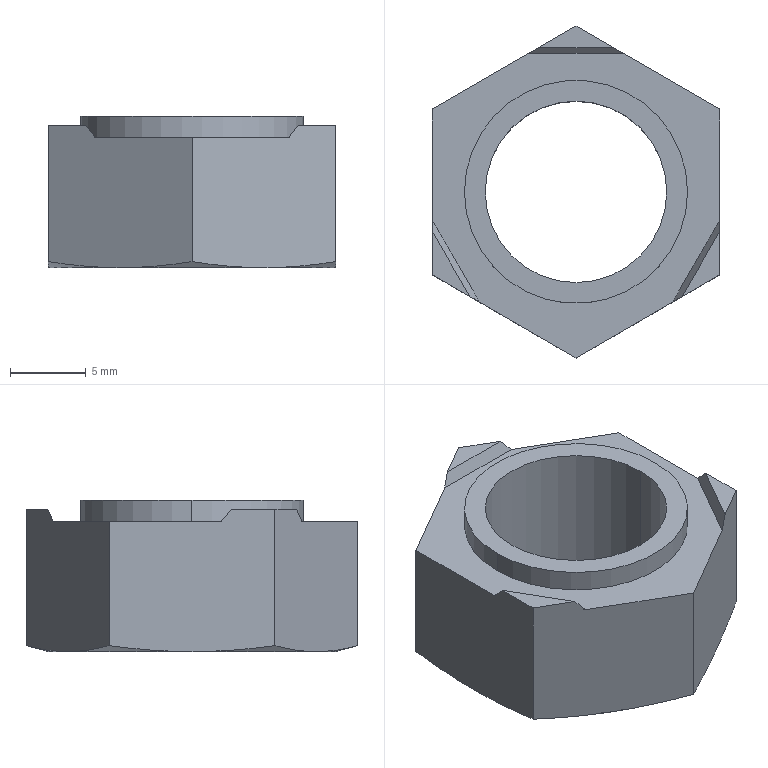Part | SolidWorks | features Cut 3, Boss 1, CirPattern 1, Extrusion 1, RefAxis 1 | 1 solid | 28 faces | box 19 x 21.939 x 10 mm | volume 1791 mm3 | plane 16 | cylinder 6 | cone 6 | commonest cylinder face diameters 12 x2 14.75 x2 15.07 x2
STEP:
#1=CARTESIAN_POINT('',(7.535,0.,0.2));
#2=VERTEX_POINT('',#1);
#3=CARTESIAN_POINT('',(-7.535,0.,0.2));
#4=VERTEX_POINT('',#3);
#5=CARTESIAN_POINT('',(0.,0.,0.2));
#6=DIRECTION('',(0.,0.,-1.));
#7=DIRECTION('',(-1.,0.,0.));
#8=AXIS2_PLACEMENT_3D('',#5,#6,#7);
#9=CIRCLE('',#8,7.535);
#10=EDGE_CURVE('',#2,#4,#9,.T.);
#11=ORIENTED_EDGE('',*,*,#10,.F.);
#12=CARTESIAN_POINT('',(7.535,0.,0.));
#13=VERTEX_POINT('',#12);
#14=CARTESIAN_POINT('',(7.535,0.,0.2));
#15=DIRECTION('',(0.,0.,-1.));
#16=VECTOR('',#15,1000.);
#17=LINE('',#14,#16);
#18=EDGE_CURVE('',#2,#13,#17,.T.);
#19=ORIENTED_EDGE('',*,*,#18,.T.);
#20=CARTESIAN_POINT('',(-7.535,0.,0.));
#21=VERTEX_POINT('',#20);
#22=CARTESIAN_POINT('',(0.,0.,0.));
#23=DIRECTION('',(0.,0.,-1.));
#24=DIRECTION('',(-1.,0.,0.));
#25=AXIS2_PLACEMENT_3D('',#22,#23,#24);
#26=CIRCLE('',#25,7.535);
#27=EDGE_CURVE('',#13,#21,#26,.T.);
#28=ORIENTED_EDGE('',*,*,#27,.T.);
#29=CARTESIAN_POINT('',(-7.535,0.,0.2));
#30=DIRECTION('',(0.,0.,-1.));
#31=VECTOR('',#30,1000.);
#32=LINE('',#29,#31);
#33=EDGE_CURVE('',#4,#21,#32,.T.);
#34=ORIENTED_EDGE('',*,*,#33,.F.);
#35=EDGE_LOOP('',(#11,#19,#28,#34));
#36=FACE_OUTER_BOUND('',#35,.T.);
#37=CARTESIAN_POINT('',(0.,0.,0.2));
#38=DIRECTION('',(0.,0.,-1.));
#39=DIRECTION('',(-1.,0.,0.));
#40=AXIS2_PLACEMENT_3D('',#37,#38,#39);
#41=CYLINDRICAL_SURFACE('',#40,7.535);
#42=ADVANCED_FACE('',(#36),#41,.F.);
#43=CARTESIAN_POINT('',(7.375,0.,10.));
#44=VERTEX_POINT('',#43);
#45=CARTESIAN_POINT('',(-7.375,0.,10.));
#46=VERTEX_POINT('',#45);
#47=CARTESIAN_POINT('',(0.,0.,10.));
#48=DIRECTION('',(0.,0.,1.));
#49=DIRECTION('',(1.,0.,0.));
#50=AXIS2_PLACEMENT_3D('',#47,#48,#49);
#51=CIRCLE('',#50,7.375);
#52=EDGE_CURVE('',#44,#46,#51,.T.);
#53=ORIENTED_EDGE('',*,*,#52,.F.);
#54=CARTESIAN_POINT('',(7.375,0.,8.6));
#55=VERTEX_POINT('',#54);
#56=CARTESIAN_POINT('',(7.375,0.,10.));
#57=DIRECTION('',(0.,0.,-1.));
#58=VECTOR('',#57,1000.);
#59=LINE('',#56,#58);
#60=EDGE_CURVE('',#44,#55,#59,.T.);
#61=ORIENTED_EDGE('',*,*,#60,.T.);
#62=CARTESIAN_POINT('',(-7.375,0.,8.6));
#63=VERTEX_POINT('',#62);
#64=CARTESIAN_POINT('',(0.,0.,8.6));
#65=DIRECTION('',(0.,0.,1.));
#66=DIRECTION('',(-1.,0.,0.));
#67=AXIS2_PLACEMENT_3D('',#64,#65,#66);
#68=CIRCLE('',#67,7.375);
#69=EDGE_CURVE('',#55,#63,#68,.T.);
#70=ORIENTED_EDGE('',*,*,#69,.T.);
#71=CARTESIAN_POINT('',(-7.375,0.,10.));
#72=DIRECTION('',(0.,0.,-1.));
#73=VECTOR('',#72,1000.);
#74=LINE('',#71,#73);
#75=EDGE_CURVE('',#46,#63,#74,.T.);
#76=ORIENTED_EDGE('',*,*,#75,.F.);
#77=EDGE_LOOP('',(#53,#61,#70,#76));
#78=FACE_OUTER_BOUND('',#77,.T.);
#79=CARTESIAN_POINT('',(0.,0.,10.));
#80=DIRECTION('',(0.,0.,-1.));
#81=DIRECTION('',(-1.,0.,0.));
#82=AXIS2_PLACEMENT_3D('',#79,#80,#81);
#83=CYLINDRICAL_SURFACE('',#82,7.375);
#84=ADVANCED_FACE('',(#78),#83,.T.);
#85=CARTESIAN_POINT('',(-6.,0.,10.));
#86=VERTEX_POINT('',#85);
#87=CARTESIAN_POINT('',(6.,0.,10.));
#88=VERTEX_POINT('',#87);
#89=CARTESIAN_POINT('',(0.,0.,10.));
#90=DIRECTION('',(0.,0.,1.));
#91=DIRECTION('',(1.,0.,0.));
#92=AXIS2_PLACEMENT_3D('',#89,#90,#91);
#93=CIRCLE('',#92,6.);
#94=EDGE_CURVE('',#86,#88,#93,.T.);
#95=ORIENTED_EDGE('',*,*,#94,.T.);
#96=CARTESIAN_POINT('',(6.,0.,0.2));
#97=VERTEX_POINT('',#96);
#98=CARTESIAN_POINT('',(6.,0.,10.));
#99=DIRECTION('',(0.,0.,-1.));
#100=VECTOR('',#99,1000.);
#101=LINE('',#98,#100);
#102=EDGE_CURVE('',#88,#97,#101,.T.);
#103=ORIENTED_EDGE('',*,*,#102,.T.);
#104=CARTESIAN_POINT('',(-6.,0.,0.2));
#105=VERTEX_POINT('',#104);
#106=CARTESIAN_POINT('',(0.,0.,0.2));
#107=DIRECTION('',(0.,0.,-1.));
#108=DIRECTION('',(-1.,0.,0.));
#109=AXIS2_PLACEMENT_3D('',#106,#107,#108);
#110=CIRCLE('',#109,6.);
#111=EDGE_CURVE('',#97,#105,#110,.T.);
#112=ORIENTED_EDGE('',*,*,#111,.T.);
#113=CARTESIAN_POINT('',(-6.,0.,10.));
#114=DIRECTION('',(0.,0.,-1.));
#115=VECTOR('',#114,1000.);
#116=LINE('',#113,#115);
#117=EDGE_CURVE('',#86,#105,#116,.T.);
#118=ORIENTED_EDGE('',*,*,#117,.F.);
#119=EDGE_LOOP('',(#95,#103,#112,#118));
#120=FACE_OUTER_BOUND('',#119,.T.);
#121=CARTESIAN_POINT('',(0.,0.,10.));
#122=DIRECTION('',(0.,0.,-1.));
#123=DIRECTION('',(-1.,0.,0.));
#124=AXIS2_PLACEMENT_3D('',#121,#122,#123);
#125=CYLINDRICAL_SURFACE('',#124,6.);
#126=ADVANCED_FACE('',(#120),#125,.F.);
#127=ORIENTED_EDGE('',*,*,#102,.F.);
#128=CARTESIAN_POINT('',(0.,0.,10.));
#129=DIRECTION('',(0.,0.,1.));
#130=DIRECTION('',(1.,0.,0.));
#131=AXIS2_PLACEMENT_3D('',#128,#129,#130);
#132=CIRCLE('',#131,6.);
#133=EDGE_CURVE('',#88,#86,#132,.T.);
#134=ORIENTED_EDGE('',*,*,#133,.T.);
#135=ORIENTED_EDGE('',*,*,#117,.T.);
#136=CARTESIAN_POINT('',(0.,0.,0.2));
#137=DIRECTION('',(0.,0.,-1.));
#138=DIRECTION('',(-1.,0.,0.));
#139=AXIS2_PLACEMENT_3D('',#136,#137,#138);
#140=CIRCLE('',#139,6.);
#141=EDGE_CURVE('',#105,#97,#140,.T.);
#142=ORIENTED_EDGE('',*,*,#141,.T.);
#143=EDGE_LOOP('',(#127,#134,#135,#142));
#144=FACE_OUTER_BOUND('',#143,.T.);
#145=CARTESIAN_POINT('',(0.,0.,10.));
#146=DIRECTION('',(0.,0.,-1.));
#147=DIRECTION('',(-1.,0.,0.));
#148=AXIS2_PLACEMENT_3D('',#145,#146,#147);
#149=CYLINDRICAL_SURFACE('',#148,6.);
#150=ADVANCED_FACE('',(#144),#149,.F.);
#151=CARTESIAN_POINT('',(0.,0.,0.));
#152=DIRECTION('',(0.,0.,-1.));
#153=DIRECTION('',(-1.,0.,0.));
#154=AXIS2_PLACEMENT_3D('',#151,#152,#153);
#155=CIRCLE('',#154,7.535);
#156=EDGE_CURVE('',#21,#13,#155,.T.);
#157=ORIENTED_EDGE('',*,*,#156,.F.);
#158=ORIENTED_EDGE('',*,*,#27,.F.);
#159=EDGE_LOOP('',(#157,#158));
#160=FACE_BOUND('',#159,.T.);
#161=CARTESIAN_POINT('',(4.75,8.227,0.));
#162=VERTEX_POINT('',#161);
#163=CARTESIAN_POINT('',(9.5,0.,0.));
#164=VERTEX_POINT('',#163);
#165=CARTESIAN_POINT('',(0.,0.,0.));
#166=DIRECTION('',(0.,0.,-1.));
#167=DIRECTION('',(-1.,0.,0.));
#168=AXIS2_PLACEMENT_3D('',#165,#166,#167);
#169=CIRCLE('',#168,9.5);
#170=EDGE_CURVE('',#162,#164,#169,.T.);
#171=ORIENTED_EDGE('',*,*,#170,.T.);
#172=CARTESIAN_POINT('',(4.75,-8.227,0.));
#173=VERTEX_POINT('',#172);
#174=CARTESIAN_POINT('',(0.,0.,0.));
#175=DIRECTION('',(0.,0.,-1.));
#176=DIRECTION('',(-1.,0.,0.));
#177=AXIS2_PLACEMENT_3D('',#174,#175,#176);
#178=CIRCLE('',#177,9.5);
#179=EDGE_CURVE('',#164,#173,#178,.T.);
#180=ORIENTED_EDGE('',*,*,#179,.T.);
#181=CARTESIAN_POINT('',(-4.75,-8.227,0.));
#182=VERTEX_POINT('',#181);
#183=CARTESIAN_POINT('',(0.,0.,0.));
#184=DIRECTION('',(0.,0.,-1.));
#185=DIRECTION('',(-1.,0.,0.));
#186=AXIS2_PLACEMENT_3D('',#183,#184,#185);
#187=CIRCLE('',#186,9.5);
#188=EDGE_CURVE('',#173,#182,#187,.T.);
#189=ORIENTED_EDGE('',*,*,#188,.T.);
#190=CARTESIAN_POINT('',(-9.5,0.,0.));
#191=VERTEX_POINT('',#190);
#192=CARTESIAN_POINT('',(0.,0.,0.));
#193=DIRECTION('',(0.,0.,-1.));
#194=DIRECTION('',(-1.,0.,0.));
#195=AXIS2_PLACEMENT_3D('',#192,#193,#194);
#196=CIRCLE('',#195,9.5);
#197=EDGE_CURVE('',#182,#191,#196,.T.);
#198=ORIENTED_EDGE('',*,*,#197,.T.);
#199=CARTESIAN_POINT('',(-4.75,8.227,0.));
#200=VERTEX_POINT('',#199);
#201=CARTESIAN_POINT('',(0.,0.,0.));
#202=DIRECTION('',(0.,0.,-1.));
#203=DIRECTION('',(-1.,0.,0.));
#204=AXIS2_PLACEMENT_3D('',#201,#202,#203);
#205=CIRCLE('',#204,9.5);
#206=EDGE_CURVE('',#191,#200,#205,.T.);
#207=ORIENTED_EDGE('',*,*,#206,.T.);
#208=CARTESIAN_POINT('',(0.,0.,0.));
#209=DIRECTION('',(0.,0.,-1.));
#210=DIRECTION('',(-1.,0.,0.));
#211=AXIS2_PLACEMENT_3D('',#208,#209,#210);
#212=CIRCLE('',#211,9.5);
#213=EDGE_CURVE('',#200,#162,#212,.T.);
#214=ORIENTED_EDGE('',*,*,#213,.T.);
#215=EDGE_LOOP('',(#171,#180,#189,#198,#207,#214));
#216=FACE_OUTER_BOUND('',#215,.T.);
#217=CARTESIAN_POINT('',(-9.5,16.454,0.));
#218=DIRECTION('',(0.,0.,1.));
#219=DIRECTION('',(1.,0.,0.));
#220=AXIS2_PLACEMENT_3D('',#217,#218,#219);
#221=PLANE('',#220);
#222=ADVANCED_FACE('',(#160,#216),#221,.F.);
#223=CARTESIAN_POINT('',(0.,10.97,0.3938));
#224=VERTEX_POINT('',#223);
#225=CARTESIAN_POINT('',(0.,10.97,0.3938));
#226=CARTESIAN_POINT('',(0.7917,10.513,0.2713));
#227=CARTESIAN_POINT('',(1.583,10.056,0.1719));
#228=CARTESIAN_POINT('',(3.167,9.141,0.03601));
#229=CARTESIAN_POINT('',(3.958,8.684,0.));
#230=CARTESIAN_POINT('',(4.75,8.227,0.));
#231=B_SPLINE_CURVE_WITH_KNOTS('',3,(#225,#226,#227,#228,#229,#230),.UNSPECIFIED.,.F.,.F.,(4,2,4),(0.000000231,0.002743,0.005485),.UNSPECIFIED.);
#232=EDGE_CURVE('',#224,#162,#231,.T.);
#233=ORIENTED_EDGE('',*,*,#232,.F.);
#234=CARTESIAN_POINT('',(0.,10.97,9.4));
#235=VERTEX_POINT('',#234);
#236=CARTESIAN_POINT('',(0.,10.97,10.));
#237=DIRECTION('',(0.,0.,-1.));
#238=VECTOR('',#237,1000.);
#239=LINE('',#236,#238);
#240=EDGE_CURVE('',#235,#224,#239,.T.);
#241=ORIENTED_EDGE('',*,*,#240,.F.);
#242=CARTESIAN_POINT('',(2.475,9.54,9.4));
#243=VERTEX_POINT('',#242);
#244=CARTESIAN_POINT('',(9.5,5.485,9.4));
#245=DIRECTION('',(0.866,-0.5,0.));
#246=VECTOR('',#245,1000.);
#247=LINE('',#244,#246);
#248=EDGE_CURVE('',#235,#243,#247,.T.);
#249=ORIENTED_EDGE('',*,*,#248,.T.);
#250=CARTESIAN_POINT('',(3.122,9.167,8.6));
#251=VERTEX_POINT('',#250);
#252=CARTESIAN_POINT('',(5.484,7.804,5.675));
#253=DIRECTION('',(0.5907,-0.341,-0.7313));
#254=VECTOR('',#253,1000.);
#255=LINE('',#252,#254);
#256=EDGE_CURVE('',#243,#251,#255,.T.);
#257=ORIENTED_EDGE('',*,*,#256,.T.);
#258=CARTESIAN_POINT('',(9.5,5.485,8.6));
#259=VERTEX_POINT('',#258);
#260=CARTESIAN_POINT('',(9.5,5.485,8.6));
#261=DIRECTION('',(0.866,-0.5,0.));
#262=VECTOR('',#261,1000.);
#263=LINE('',#260,#262);
#264=EDGE_CURVE('',#251,#259,#263,.T.);
#265=ORIENTED_EDGE('',*,*,#264,.T.);
#266=CARTESIAN_POINT('',(9.5,5.485,0.3938));
#267=VERTEX_POINT('',#266);
#268=CARTESIAN_POINT('',(9.5,5.485,10.));
#269=DIRECTION('',(0.,0.,-1.));
#270=VECTOR('',#269,1000.);
#271=LINE('',#268,#270);
#272=EDGE_CURVE('',#259,#267,#271,.T.);
#273=ORIENTED_EDGE('',*,*,#272,.T.);
#274=CARTESIAN_POINT('',(4.75,8.227,0.));
#275=CARTESIAN_POINT('',(5.542,7.77,0.));
#276=CARTESIAN_POINT('',(6.333,7.313,0.03601));
#277=CARTESIAN_POINT('',(7.917,6.399,0.1719));
#278=CARTESIAN_POINT('',(8.708,5.942,0.2713));
#279=CARTESIAN_POINT('',(9.5,5.485,0.3938));
#280=B_SPLINE_CURVE_WITH_KNOTS('',3,(#274,#275,#276,#277,#278,#279),.UNSPECIFIED.,.F.,.F.,(4,2,4),(0.005485,0.008227,0.01097),.UNSPECIFIED.);
#281=EDGE_CURVE('',#162,#267,#280,.T.);
#282=ORIENTED_EDGE('',*,*,#281,.F.);
#283=EDGE_LOOP('',(#233,#241,#249,#257,#265,#273,#282));
#284=FACE_OUTER_BOUND('',#283,.T.);
#285=CARTESIAN_POINT('',(9.5,5.485,10.));
#286=DIRECTION('',(-0.5,-0.866,0.));
#287=DIRECTION('',(0.866,-0.5,0.));
#288=AXIS2_PLACEMENT_3D('',#285,#286,#287);
#289=PLANE('',#288);
#290=ADVANCED_FACE('',(#284),#289,.F.);
#291=CARTESIAN_POINT('',(-9.5,5.485,0.3938));
#292=VERTEX_POINT('',#291);
#293=CARTESIAN_POINT('',(-9.5,5.485,0.3938));
#294=CARTESIAN_POINT('',(-8.708,5.942,0.2713));
#295=CARTESIAN_POINT('',(-7.917,6.399,0.1719));
#296=CARTESIAN_POINT('',(-6.333,7.313,0.03601));
#297=CARTESIAN_POINT('',(-5.542,7.77,0.));
#298=CARTESIAN_POINT('',(-4.75,8.227,0.));
#299=B_SPLINE_CURVE_WITH_KNOTS('',3,(#293,#294,#295,#296,#297,#298),.UNSPECIFIED.,.F.,.F.,(4,2,4),(0.000000231,0.002743,0.005485),.UNSPECIFIED.);
#300=EDGE_CURVE('',#292,#200,#299,.T.);
#301=ORIENTED_EDGE('',*,*,#300,.F.);
#302=CARTESIAN_POINT('',(-9.5,5.485,8.6));
#303=VERTEX_POINT('',#302);
#304=CARTESIAN_POINT('',(-9.5,5.485,10.));
#305=DIRECTION('',(0.,0.,-1.));
#306=VECTOR('',#305,1000.);
#307=LINE('',#304,#306);
#308=EDGE_CURVE('',#303,#292,#307,.T.);
#309=ORIENTED_EDGE('',*,*,#308,.F.);
#310=CARTESIAN_POINT('',(-3.122,9.167,8.6));
#311=VERTEX_POINT('',#310);
#312=CARTESIAN_POINT('',(0.,10.97,8.6));
#313=DIRECTION('',(0.866,0.5,0.));
#314=VECTOR('',#313,1000.);
#315=LINE('',#312,#314);
#316=EDGE_CURVE('',#303,#311,#315,.T.);
#317=ORIENTED_EDGE('',*,*,#316,.T.);
#318=CARTESIAN_POINT('',(-2.475,9.54,9.4));
#319=VERTEX_POINT('',#318);
#320=CARTESIAN_POINT('',(-1.065,10.355,11.147));
#321=DIRECTION('',(0.5907,0.341,0.7313));
#322=VECTOR('',#321,1000.);
#323=LINE('',#320,#322);
#324=EDGE_CURVE('',#311,#319,#323,.T.);
#325=ORIENTED_EDGE('',*,*,#324,.T.);
#326=CARTESIAN_POINT('',(0.,10.97,9.4));
#327=DIRECTION('',(0.866,0.5,0.));
#328=VECTOR('',#327,1000.);
#329=LINE('',#326,#328);
#330=EDGE_CURVE('',#319,#235,#329,.T.);
#331=ORIENTED_EDGE('',*,*,#330,.T.);
#332=ORIENTED_EDGE('',*,*,#240,.T.);
#333=CARTESIAN_POINT('',(-4.75,8.227,0.));
#334=CARTESIAN_POINT('',(-3.958,8.684,0.));
#335=CARTESIAN_POINT('',(-3.167,9.141,0.03601));
#336=CARTESIAN_POINT('',(-1.583,10.056,0.1719));
#337=CARTESIAN_POINT('',(-0.7917,10.513,0.2713));
#338=CARTESIAN_POINT('',(0.,10.97,0.3938));
#339=B_SPLINE_CURVE_WITH_KNOTS('',3,(#333,#334,#335,#336,#337,#338),.UNSPECIFIED.,.F.,.F.,(4,2,4),(0.005485,0.008227,0.01097),.UNSPECIFIED.);
#340=EDGE_CURVE('',#200,#224,#339,.T.);
#341=ORIENTED_EDGE('',*,*,#340,.F.);
#342=EDGE_LOOP('',(#301,#309,#317,#325,#331,#332,#341));
#343=FACE_OUTER_BOUND('',#342,.T.);
#344=CARTESIAN_POINT('',(0.,10.97,10.));
#345=DIRECTION('',(0.5,-0.866,0.));
#346=DIRECTION('',(0.866,0.5,0.));
#347=AXIS2_PLACEMENT_3D('',#344,#345,#346);
#348=PLANE('',#347);
#349=ADVANCED_FACE('',(#343),#348,.F.);
#350=CARTESIAN_POINT('',(-9.5,-5.485,0.3938));
#351=VERTEX_POINT('',#350);
#352=CARTESIAN_POINT('',(-9.5,-5.485,0.3938));
#353=CARTESIAN_POINT('',(-9.5,-4.573,0.2717));
#354=CARTESIAN_POINT('',(-9.5,-3.656,0.1718));
#355=CARTESIAN_POINT('',(-9.5,-1.827,0.03592));
#356=CARTESIAN_POINT('',(-9.5,-0.9129,0.));
#357=CARTESIAN_POINT('',(-9.5,0.,0.));
#358=B_SPLINE_CURVE_WITH_KNOTS('',3,(#352,#353,#354,#355,#356,#357),.UNSPECIFIED.,.F.,.F.,(4,2,4),(0.009321,0.01208,0.01483),.UNSPECIFIED.);
#359=EDGE_CURVE('',#351,#191,#358,.T.);
#360=ORIENTED_EDGE('',*,*,#359,.F.);
#361=CARTESIAN_POINT('',(-9.5,-5.485,9.4));
#362=VERTEX_POINT('',#361);
#363=CARTESIAN_POINT('',(-9.5,-5.485,10.));
#364=DIRECTION('',(0.,0.,-1.));
#365=VECTOR('',#364,1000.);
#366=LINE('',#363,#365);
#367=EDGE_CURVE('',#362,#351,#366,.T.);
#368=ORIENTED_EDGE('',*,*,#367,.F.);
#369=CARTESIAN_POINT('',(-9.5,-2.627,9.4));
#370=VERTEX_POINT('',#369);
#371=CARTESIAN_POINT('',(-9.5,5.485,9.4));
#372=DIRECTION('',(0.,1.,0.));
#373=VECTOR('',#372,1000.);
#374=LINE('',#371,#373);
#375=EDGE_CURVE('',#362,#370,#374,.T.);
#376=ORIENTED_EDGE('',*,*,#375,.T.);
#377=CARTESIAN_POINT('',(-9.5,-1.88,8.6));
#378=VERTEX_POINT('',#377);
#379=CARTESIAN_POINT('',(-9.5,0.8474,5.675));
#380=DIRECTION('',(0.,0.682,-0.7313));
#381=VECTOR('',#380,1000.);
#382=LINE('',#379,#381);
#383=EDGE_CURVE('',#370,#378,#382,.T.);
#384=ORIENTED_EDGE('',*,*,#383,.T.);
#385=CARTESIAN_POINT('',(-9.5,0.,8.6));
#386=DIRECTION('',(0.,1.,0.));
#387=VECTOR('',#386,1000.);
#388=LINE('',#385,#387);
#389=EDGE_CURVE('',#378,#303,#388,.T.);
#390=ORIENTED_EDGE('',*,*,#389,.T.);
#391=ORIENTED_EDGE('',*,*,#308,.T.);
#392=CARTESIAN_POINT('',(-9.5,0.,0.));
#393=CARTESIAN_POINT('',(-9.5,0.9159,0.));
#394=CARTESIAN_POINT('',(-9.5,1.831,0.03614));
#395=CARTESIAN_POINT('',(-9.5,3.659,0.1721));
#396=CARTESIAN_POINT('',(-9.5,4.572,0.2715));
#397=CARTESIAN_POINT('',(-9.5,5.485,0.3938));
#398=B_SPLINE_CURVE_WITH_KNOTS('',3,(#392,#393,#394,#395,#396,#397),.UNSPECIFIED.,.F.,.F.,(4,2,4),(0.01483,0.0176,0.02036),.UNSPECIFIED.);
#399=EDGE_CURVE('',#191,#292,#398,.T.);
#400=ORIENTED_EDGE('',*,*,#399,.F.);
#401=EDGE_LOOP('',(#360,#368,#376,#384,#390,#391,#400));
#402=FACE_OUTER_BOUND('',#401,.T.);
#403=CARTESIAN_POINT('',(-9.5,5.485,10.));
#404=DIRECTION('',(1.,0.,0.));
#405=DIRECTION('',(0.,0.,-1.));
#406=AXIS2_PLACEMENT_3D('',#403,#404,#405);
#407=PLANE('',#406);
#408=ADVANCED_FACE('',(#402),#407,.F.);
#409=CARTESIAN_POINT('',(0.,-10.97,0.3938));
#410=VERTEX_POINT('',#409);
#411=CARTESIAN_POINT('',(0.,-10.97,0.3938));
#412=CARTESIAN_POINT('',(-0.7917,-10.513,0.2713));
#413=CARTESIAN_POINT('',(-1.583,-10.056,0.1719));
#414=CARTESIAN_POINT('',(-3.167,-9.141,0.03601));
#415=CARTESIAN_POINT('',(-3.958,-8.684,0.));
#416=CARTESIAN_POINT('',(-4.75,-8.227,0.));
#417=B_SPLINE_CURVE_WITH_KNOTS('',3,(#411,#412,#413,#414,#415,#416),.UNSPECIFIED.,.F.,.F.,(4,2,4),(0.000000231,0.002743,0.005485),.UNSPECIFIED.);
#418=EDGE_CURVE('',#410,#182,#417,.T.);
#419=ORIENTED_EDGE('',*,*,#418,.F.);
#420=CARTESIAN_POINT('',(0.,-10.97,8.6));
#421=VERTEX_POINT('',#420);
#422=CARTESIAN_POINT('',(0.,-10.97,10.));
#423=DIRECTION('',(0.,0.,-1.));
#424=VECTOR('',#423,1000.);
#425=LINE('',#422,#424);
#426=EDGE_CURVE('',#421,#410,#425,.T.);
#427=ORIENTED_EDGE('',*,*,#426,.F.);
#428=CARTESIAN_POINT('',(-6.378,-7.287,8.6));
#429=VERTEX_POINT('',#428);
#430=CARTESIAN_POINT('',(-9.5,-5.485,8.6));
#431=DIRECTION('',(-0.866,0.5,0.));
#432=VECTOR('',#431,1000.);
#433=LINE('',#430,#432);
#434=EDGE_CURVE('',#421,#429,#433,.T.);
#435=ORIENTED_EDGE('',*,*,#434,.T.);
#436=CARTESIAN_POINT('',(-7.025,-6.914,9.4));
#437=VERTEX_POINT('',#436);
#438=CARTESIAN_POINT('',(-8.435,-6.1,11.147));
#439=DIRECTION('',(-0.5907,0.341,0.7313));
#440=VECTOR('',#439,1000.);
#441=LINE('',#438,#440);
#442=EDGE_CURVE('',#429,#437,#441,.T.);
#443=ORIENTED_EDGE('',*,*,#442,.T.);
#444=CARTESIAN_POINT('',(-9.5,-5.485,9.4));
#445=DIRECTION('',(-0.866,0.5,0.));
#446=VECTOR('',#445,1000.);
#447=LINE('',#444,#446);
#448=EDGE_CURVE('',#437,#362,#447,.T.);
#449=ORIENTED_EDGE('',*,*,#448,.T.);
#450=ORIENTED_EDGE('',*,*,#367,.T.);
#451=CARTESIAN_POINT('',(-4.75,-8.227,0.));
#452=CARTESIAN_POINT('',(-5.542,-7.77,0.));
#453=CARTESIAN_POINT('',(-6.333,-7.313,0.03601));
#454=CARTESIAN_POINT('',(-7.917,-6.399,0.1719));
#455=CARTESIAN_POINT('',(-8.708,-5.942,0.2713));
#456=CARTESIAN_POINT('',(-9.5,-5.485,0.3938));
#457=B_SPLINE_CURVE_WITH_KNOTS('',3,(#451,#452,#453,#454,#455,#456),.UNSPECIFIED.,.F.,.F.,(4,2,4),(0.005485,0.008227,0.01097),.UNSPECIFIED.);
#458=EDGE_CURVE('',#182,#351,#457,.T.);
#459=ORIENTED_EDGE('',*,*,#458,.F.);
#460=EDGE_LOOP('',(#419,#427,#435,#443,#449,#450,#459));
#461=FACE_OUTER_BOUND('',#460,.T.);
#462=CARTESIAN_POINT('',(-9.5,-5.485,10.));
#463=DIRECTION('',(0.5,0.866,0.));
#464=DIRECTION('',(-0.866,0.5,0.));
#465=AXIS2_PLACEMENT_3D('',#462,#463,#464);
#466=PLANE('',#465);
#467=ADVANCED_FACE('',(#461),#466,.F.);
#468=CARTESIAN_POINT('',(9.5,-5.485,0.3938));
#469=VERTEX_POINT('',#468);
#470=CARTESIAN_POINT('',(9.5,-5.485,0.3938));
#471=CARTESIAN_POINT('',(8.708,-5.942,0.2713));
#472=CARTESIAN_POINT('',(7.917,-6.399,0.1719));
#473=CARTESIAN_POINT('',(6.333,-7.313,0.03601));
#474=CARTESIAN_POINT('',(5.542,-7.77,0.));
#475=CARTESIAN_POINT('',(4.75,-8.227,0.));
#476=B_SPLINE_CURVE_WITH_KNOTS('',3,(#470,#471,#472,#473,#474,#475),.UNSPECIFIED.,.F.,.F.,(4,2,4),(0.000000231,0.002743,0.005485),.UNSPECIFIED.);
#477=EDGE_CURVE('',#469,#173,#476,.T.);
#478=ORIENTED_EDGE('',*,*,#477,.F.);
#479=CARTESIAN_POINT('',(9.5,-5.485,9.4));
#480=VERTEX_POINT('',#479);
#481=CARTESIAN_POINT('',(9.5,-5.485,10.));
#482=DIRECTION('',(0.,0.,-1.));
#483=VECTOR('',#482,1000.);
#484=LINE('',#481,#483);
#485=EDGE_CURVE('',#480,#469,#484,.T.);
#486=ORIENTED_EDGE('',*,*,#485,.F.);
#487=CARTESIAN_POINT('',(7.025,-6.914,9.4));
#488=VERTEX_POINT('',#487);
#489=CARTESIAN_POINT('',(0.,-10.97,9.4));
#490=DIRECTION('',(-0.866,-0.5,0.));
#491=VECTOR('',#490,1000.);
#492=LINE('',#489,#491);
#493=EDGE_CURVE('',#480,#488,#492,.T.);
#494=ORIENTED_EDGE('',*,*,#493,.T.);
#495=CARTESIAN_POINT('',(6.378,-7.287,8.6));
#496=VERTEX_POINT('',#495);
#497=CARTESIAN_POINT('',(4.016,-8.651,5.675));
#498=DIRECTION('',(-0.5907,-0.341,-0.7313));
#499=VECTOR('',#498,1000.);
#500=LINE('',#497,#499);
#501=EDGE_CURVE('',#488,#496,#500,.T.);
#502=ORIENTED_EDGE('',*,*,#501,.T.);
#503=CARTESIAN_POINT('',(0.,-10.97,8.6));
#504=DIRECTION('',(-0.866,-0.5,0.));
#505=VECTOR('',#504,1000.);
#506=LINE('',#503,#505);
#507=EDGE_CURVE('',#496,#421,#506,.T.);
#508=ORIENTED_EDGE('',*,*,#507,.T.);
#509=ORIENTED_EDGE('',*,*,#426,.T.);
#510=CARTESIAN_POINT('',(4.75,-8.227,0.));
#511=CARTESIAN_POINT('',(3.958,-8.684,0.));
#512=CARTESIAN_POINT('',(3.167,-9.141,0.03601));
#513=CARTESIAN_POINT('',(1.583,-10.056,0.1719));
#514=CARTESIAN_POINT('',(0.7917,-10.513,0.2713));
#515=CARTESIAN_POINT('',(0.,-10.97,0.3938));
#516=B_SPLINE_CURVE_WITH_KNOTS('',3,(#510,#511,#512,#513,#514,#515),.UNSPECIFIED.,.F.,.F.,(4,2,4),(0.005485,0.008227,0.01097),.UNSPECIFIED.);
#517=EDGE_CURVE('',#173,#410,#516,.T.);
#518=ORIENTED_EDGE('',*,*,#517,.F.);
#519=EDGE_LOOP('',(#478,#486,#494,#502,#508,#509,#518));
#520=FACE_OUTER_BOUND('',#519,.T.);
#521=CARTESIAN_POINT('',(0.,-10.97,10.));
#522=DIRECTION('',(-0.5,0.866,0.));
#523=DIRECTION('',(-0.866,-0.5,0.));
#524=AXIS2_PLACEMENT_3D('',#521,#522,#523);
#525=PLANE('',#524);
#526=ADVANCED_FACE('',(#520),#525,.F.);
#527=CARTESIAN_POINT('',(9.5,5.485,0.3938));
#528=CARTESIAN_POINT('',(9.5,4.572,0.2715));
#529=CARTESIAN_POINT('',(9.5,3.659,0.1721));
#530=CARTESIAN_POINT('',(9.5,1.831,0.03614));
#531=CARTESIAN_POINT('',(9.5,0.9159,0.));
#532=CARTESIAN_POINT('',(9.5,0.,0.));
#533=B_SPLINE_CURVE_WITH_KNOTS('',3,(#527,#528,#529,#530,#531,#532),.UNSPECIFIED.,.F.,.F.,(4,2,4),(0.02789,0.03065,0.03341),.UNSPECIFIED.);
#534=EDGE_CURVE('',#267,#164,#533,.T.);
#535=ORIENTED_EDGE('',*,*,#534,.F.);
#536=ORIENTED_EDGE('',*,*,#272,.F.);
#537=CARTESIAN_POINT('',(9.5,-1.88,8.6));
#538=VERTEX_POINT('',#537);
#539=CARTESIAN_POINT('',(9.5,0.,8.6));
#540=DIRECTION('',(0.,1.,0.));
#541=VECTOR('',#540,1000.);
#542=LINE('',#539,#541);
#543=EDGE_CURVE('',#538,#259,#542,.T.);
#544=ORIENTED_EDGE('',*,*,#543,.F.);
#545=CARTESIAN_POINT('',(9.5,-2.627,9.4));
#546=VERTEX_POINT('',#545);
#547=CARTESIAN_POINT('',(9.5,-4.255,11.147));
#548=DIRECTION('',(0.,-0.682,0.7313));
#549=VECTOR('',#548,1000.);
#550=LINE('',#547,#549);
#551=EDGE_CURVE('',#538,#546,#550,.T.);
#552=ORIENTED_EDGE('',*,*,#551,.T.);
#553=CARTESIAN_POINT('',(9.5,-5.485,9.4));
#554=DIRECTION('',(0.,-1.,0.));
#555=VECTOR('',#554,1000.);
#556=LINE('',#553,#555);
#557=EDGE_CURVE('',#546,#480,#556,.T.);
#558=ORIENTED_EDGE('',*,*,#557,.T.);
#559=ORIENTED_EDGE('',*,*,#485,.T.);
#560=CARTESIAN_POINT('',(9.5,0.,0.));
#561=CARTESIAN_POINT('',(9.5,-0.9129,0.));
#562=CARTESIAN_POINT('',(9.5,-1.827,0.03592));
#563=CARTESIAN_POINT('',(9.5,-3.656,0.1718));
#564=CARTESIAN_POINT('',(9.5,-4.573,0.2717));
#565=CARTESIAN_POINT('',(9.5,-5.485,0.3938));
#566=B_SPLINE_CURVE_WITH_KNOTS('',3,(#560,#561,#562,#563,#564,#565),.UNSPECIFIED.,.F.,.F.,(4,2,4),(0.03341,0.03616,0.03891),.UNSPECIFIED.);
#567=EDGE_CURVE('',#164,#469,#566,.T.);
#568=ORIENTED_EDGE('',*,*,#567,.F.);
#569=EDGE_LOOP('',(#535,#536,#544,#552,#558,#559,#568));
#570=FACE_OUTER_BOUND('',#569,.T.);
#571=CARTESIAN_POINT('',(9.5,-5.485,10.));
#572=DIRECTION('',(-1.,0.,0.));
#573=DIRECTION('',(0.,0.,1.));
#574=AXIS2_PLACEMENT_3D('',#571,#572,#573);
#575=PLANE('',#574);
#576=ADVANCED_FACE('',(#570),#575,.F.);
#577=CARTESIAN_POINT('',(-9.5,9.167,8.6));
#578=DIRECTION('',(1.,0.,0.));
#579=VECTOR('',#578,1000.);
#580=LINE('',#577,#579);
#581=EDGE_CURVE('',#311,#251,#580,.T.);
#582=ORIENTED_EDGE('',*,*,#581,.F.);
#583=ORIENTED_EDGE('',*,*,#316,.F.);
#584=ORIENTED_EDGE('',*,*,#389,.F.);
#585=CARTESIAN_POINT('',(-0.8142,-16.925,8.6));
#586=DIRECTION('',(-0.5,0.866,0.));
#587=VECTOR('',#586,1000.);
#588=LINE('',#585,#587);
#589=EDGE_CURVE('',#429,#378,#588,.T.);
#590=ORIENTED_EDGE('',*,*,#589,.F.);
#591=ORIENTED_EDGE('',*,*,#434,.F.);
#592=ORIENTED_EDGE('',*,*,#507,.F.);
#593=CARTESIAN_POINT('',(15.064,7.757,8.6));
#594=DIRECTION('',(-0.5,-0.866,0.));
#595=VECTOR('',#594,1000.);
#596=LINE('',#593,#595);
#597=EDGE_CURVE('',#538,#496,#596,.T.);
#598=ORIENTED_EDGE('',*,*,#597,.F.);
#599=ORIENTED_EDGE('',*,*,#543,.T.);
#600=ORIENTED_EDGE('',*,*,#264,.F.);
#601=EDGE_LOOP('',(#582,#583,#584,#590,#591,#592,#598,#599,#600));
#602=FACE_OUTER_BOUND('',#601,.T.);
#603=CARTESIAN_POINT('',(0.,0.,8.6));
#604=DIRECTION('',(0.,0.,1.));
#605=DIRECTION('',(-1.,0.,0.));
#606=AXIS2_PLACEMENT_3D('',#603,#604,#605);
#607=CIRCLE('',#606,7.375);
#608=EDGE_CURVE('',#63,#55,#607,.T.);
#609=ORIENTED_EDGE('',*,*,#608,.F.);
#610=ORIENTED_EDGE('',*,*,#69,.F.);
#611=EDGE_LOOP('',(#609,#610));
#612=FACE_BOUND('',#611,.T.);
#613=CARTESIAN_POINT('',(-9.5,0.,8.6));
#614=DIRECTION('',(0.,0.,-1.));
#615=DIRECTION('',(-1.,0.,0.));
#616=AXIS2_PLACEMENT_3D('',#613,#614,#615);
#617=PLANE('',#616);
#618=ADVANCED_FACE('',(#602,#612),#617,.F.);
#619=ORIENTED_EDGE('',*,*,#330,.F.);
#620=CARTESIAN_POINT('',(-9.5,9.54,9.4));
#621=DIRECTION('',(1.,0.,0.));
#622=VECTOR('',#621,1000.);
#623=LINE('',#620,#622);
#624=EDGE_CURVE('',#319,#243,#623,.T.);
#625=ORIENTED_EDGE('',*,*,#624,.T.);
#626=ORIENTED_EDGE('',*,*,#248,.F.);
#627=EDGE_LOOP('',(#619,#625,#626));
#628=FACE_OUTER_BOUND('',#627,.T.);
#629=CARTESIAN_POINT('',(-9.5,9.54,9.4));
#630=DIRECTION('',(0.,0.,-1.));
#631=DIRECTION('',(-1.,0.,0.));
#632=AXIS2_PLACEMENT_3D('',#629,#630,#631);
#633=PLANE('',#632);
#634=ADVANCED_FACE('',(#628),#633,.F.);
#635=ORIENTED_EDGE('',*,*,#624,.F.);
#636=ORIENTED_EDGE('',*,*,#324,.F.);
#637=ORIENTED_EDGE('',*,*,#581,.T.);
#638=ORIENTED_EDGE('',*,*,#256,.F.);
#639=EDGE_LOOP('',(#635,#636,#637,#638));
#640=FACE_OUTER_BOUND('',#639,.T.);
#641=CARTESIAN_POINT('',(-9.5,9.54,9.4));
#642=DIRECTION('',(0.,0.9063,-0.4226));
#643=DIRECTION('',(0.,0.4226,0.9063));
#644=AXIS2_PLACEMENT_3D('',#641,#642,#643);
#645=PLANE('',#644);
#646=ADVANCED_FACE('',(#640),#645,.F.);
#647=ORIENTED_EDGE('',*,*,#448,.F.);
#648=CARTESIAN_POINT('',(-1.137,-17.111,9.4));
#649=DIRECTION('',(-0.5,0.866,0.));
#650=VECTOR('',#649,1000.);
#651=LINE('',#648,#650);
#652=EDGE_CURVE('',#437,#370,#651,.T.);
#653=ORIENTED_EDGE('',*,*,#652,.T.);
#654=ORIENTED_EDGE('',*,*,#375,.F.);
#655=EDGE_LOOP('',(#647,#653,#654));
#656=FACE_OUTER_BOUND('',#655,.T.);
#657=CARTESIAN_POINT('',(-1.137,-17.111,9.4));
#658=DIRECTION('',(0.,0.,-1.));
#659=DIRECTION('',(-1.,0.,0.));
#660=AXIS2_PLACEMENT_3D('',#657,#658,#659);
#661=PLANE('',#660);
#662=ADVANCED_FACE('',(#656),#661,.F.);
#663=ORIENTED_EDGE('',*,*,#652,.F.);
#664=ORIENTED_EDGE('',*,*,#442,.F.);
#665=ORIENTED_EDGE('',*,*,#589,.T.);
#666=ORIENTED_EDGE('',*,*,#383,.F.);
#667=EDGE_LOOP('',(#663,#664,#665,#666));
#668=FACE_OUTER_BOUND('',#667,.T.);
#669=CARTESIAN_POINT('',(-1.137,-17.111,9.4));
#670=DIRECTION('',(-0.7849,-0.4532,-0.4226));
#671=DIRECTION('',(0.5,-0.866,0.));
#672=AXIS2_PLACEMENT_3D('',#669,#670,#671);
#673=PLANE('',#672);
#674=ADVANCED_FACE('',(#668),#673,.F.);
#675=ORIENTED_EDGE('',*,*,#557,.F.);
#676=CARTESIAN_POINT('',(15.387,7.571,9.4));
#677=DIRECTION('',(-0.5,-0.866,0.));
#678=VECTOR('',#677,1000.);
#679=LINE('',#676,#678);
#680=EDGE_CURVE('',#546,#488,#679,.T.);
#681=ORIENTED_EDGE('',*,*,#680,.T.);
#682=ORIENTED_EDGE('',*,*,#493,.F.);
#683=EDGE_LOOP('',(#675,#681,#682));
#684=FACE_OUTER_BOUND('',#683,.T.);
#685=CARTESIAN_POINT('',(15.387,7.571,9.4));
#686=DIRECTION('',(0.,0.,-1.));
#687=DIRECTION('',(-1.,0.,0.));
#688=AXIS2_PLACEMENT_3D('',#685,#686,#687);
#689=PLANE('',#688);
#690=ADVANCED_FACE('',(#684),#689,.F.);
#691=ORIENTED_EDGE('',*,*,#680,.F.);
#692=ORIENTED_EDGE('',*,*,#551,.F.);
#693=ORIENTED_EDGE('',*,*,#597,.T.);
#694=ORIENTED_EDGE('',*,*,#501,.F.);
#695=EDGE_LOOP('',(#691,#692,#693,#694));
#696=FACE_OUTER_BOUND('',#695,.T.);
#697=CARTESIAN_POINT('',(15.387,7.571,9.4));
#698=DIRECTION('',(0.7849,-0.4532,-0.4226));
#699=DIRECTION('',(0.5,0.866,0.));
#700=AXIS2_PLACEMENT_3D('',#697,#698,#699);
#701=PLANE('',#700);
#702=ADVANCED_FACE('',(#696),#701,.F.);
#703=CARTESIAN_POINT('',(0.,0.,10.));
#704=DIRECTION('',(0.,0.,1.));
#705=DIRECTION('',(1.,0.,0.));
#706=AXIS2_PLACEMENT_3D('',#703,#704,#705);
#707=CIRCLE('',#706,7.375);
#708=EDGE_CURVE('',#46,#44,#707,.T.);
#709=ORIENTED_EDGE('',*,*,#708,.T.);
#710=ORIENTED_EDGE('',*,*,#52,.T.);
#711=EDGE_LOOP('',(#709,#710));
#712=FACE_OUTER_BOUND('',#711,.T.);
#713=ORIENTED_EDGE('',*,*,#94,.F.);
#714=ORIENTED_EDGE('',*,*,#133,.F.);
#715=EDGE_LOOP('',(#713,#714));
#716=FACE_BOUND('',#715,.T.);
#717=CARTESIAN_POINT('',(0.,0.,10.));
#718=DIRECTION('',(0.,0.,1.));
#719=DIRECTION('',(1.,0.,0.));
#720=AXIS2_PLACEMENT_3D('',#717,#718,#719);
#721=PLANE('',#720);
#722=ADVANCED_FACE('',(#712,#716),#721,.T.);
#723=ORIENTED_EDGE('',*,*,#60,.F.);
#724=ORIENTED_EDGE('',*,*,#708,.F.);
#725=ORIENTED_EDGE('',*,*,#75,.T.);
#726=ORIENTED_EDGE('',*,*,#608,.T.);
#727=EDGE_LOOP('',(#723,#724,#725,#726));
#728=FACE_OUTER_BOUND('',#727,.T.);
#729=CARTESIAN_POINT('',(0.,0.,10.));
#730=DIRECTION('',(0.,0.,-1.));
#731=DIRECTION('',(-1.,0.,0.));
#732=AXIS2_PLACEMENT_3D('',#729,#730,#731);
#733=CYLINDRICAL_SURFACE('',#732,7.375);
#734=ADVANCED_FACE('',(#728),#733,.T.);
#735=ORIENTED_EDGE('',*,*,#477,.T.);
#736=ORIENTED_EDGE('',*,*,#179,.F.);
#737=ORIENTED_EDGE('',*,*,#567,.T.);
#738=EDGE_LOOP('',(#735,#736,#737));
#739=FACE_OUTER_BOUND('',#738,.T.);
#740=CARTESIAN_POINT('',(0.,0.,0.));
#741=DIRECTION('',(0.,0.,1.));
#742=DIRECTION('',(-1.,0.,0.));
#743=AXIS2_PLACEMENT_3D('',#740,#741,#742);
#744=CONICAL_SURFACE('',#743,9.5,1.309);
#745=ADVANCED_FACE('',(#739),#744,.T.);
#746=ORIENTED_EDGE('',*,*,#281,.T.);
#747=ORIENTED_EDGE('',*,*,#534,.T.);
#748=ORIENTED_EDGE('',*,*,#170,.F.);
#749=EDGE_LOOP('',(#746,#747,#748));
#750=FACE_OUTER_BOUND('',#749,.T.);
#751=CARTESIAN_POINT('',(0.,0.,0.));
#752=DIRECTION('',(0.,0.,1.));
#753=DIRECTION('',(-1.,0.,0.));
#754=AXIS2_PLACEMENT_3D('',#751,#752,#753);
#755=CONICAL_SURFACE('',#754,9.5,1.309);
#756=ADVANCED_FACE('',(#750),#755,.T.);
#757=ORIENTED_EDGE('',*,*,#418,.T.);
#758=ORIENTED_EDGE('',*,*,#188,.F.);
#759=ORIENTED_EDGE('',*,*,#517,.T.);
#760=EDGE_LOOP('',(#757,#758,#759));
#761=FACE_OUTER_BOUND('',#760,.T.);
#762=CARTESIAN_POINT('',(0.,0.,0.));
#763=DIRECTION('',(0.,0.,1.));
#764=DIRECTION('',(-1.,0.,0.));
#765=AXIS2_PLACEMENT_3D('',#762,#763,#764);
#766=CONICAL_SURFACE('',#765,9.5,1.309);
#767=ADVANCED_FACE('',(#761),#766,.T.);
#768=ORIENTED_EDGE('',*,*,#359,.T.);
#769=ORIENTED_EDGE('',*,*,#197,.F.);
#770=ORIENTED_EDGE('',*,*,#458,.T.);
#771=EDGE_LOOP('',(#768,#769,#770));
#772=FACE_OUTER_BOUND('',#771,.T.);
#773=CARTESIAN_POINT('',(0.,0.,0.));
#774=DIRECTION('',(0.,0.,1.));
#775=DIRECTION('',(-1.,0.,0.));
#776=AXIS2_PLACEMENT_3D('',#773,#774,#775);
#777=CONICAL_SURFACE('',#776,9.5,1.309);
#778=ADVANCED_FACE('',(#772),#777,.T.);
#779=ORIENTED_EDGE('',*,*,#399,.T.);
#780=ORIENTED_EDGE('',*,*,#300,.T.);
#781=ORIENTED_EDGE('',*,*,#206,.F.);
#782=EDGE_LOOP('',(#779,#780,#781));
#783=FACE_OUTER_BOUND('',#782,.T.);
#784=CARTESIAN_POINT('',(0.,0.,0.));
#785=DIRECTION('',(0.,0.,1.));
#786=DIRECTION('',(-1.,0.,0.));
#787=AXIS2_PLACEMENT_3D('',#784,#785,#786);
#788=CONICAL_SURFACE('',#787,9.5,1.309);
#789=ADVANCED_FACE('',(#783),#788,.T.);
#790=ORIENTED_EDGE('',*,*,#340,.T.);
#791=ORIENTED_EDGE('',*,*,#232,.T.);
#792=ORIENTED_EDGE('',*,*,#213,.F.);
#793=EDGE_LOOP('',(#790,#791,#792));
#794=FACE_OUTER_BOUND('',#793,.T.);
#795=CARTESIAN_POINT('',(0.,0.,0.));
#796=DIRECTION('',(0.,0.,1.));
#797=DIRECTION('',(-1.,0.,0.));
#798=AXIS2_PLACEMENT_3D('',#795,#796,#797);
#799=CONICAL_SURFACE('',#798,9.5,1.309);
#800=ADVANCED_FACE('',(#794),#799,.T.);
#801=ORIENTED_EDGE('',*,*,#18,.F.);
#802=CARTESIAN_POINT('',(0.,0.,0.2));
#803=DIRECTION('',(0.,0.,-1.));
#804=DIRECTION('',(-1.,0.,0.));
#805=AXIS2_PLACEMENT_3D('',#802,#803,#804);
#806=CIRCLE('',#805,7.535);
#807=EDGE_CURVE('',#4,#2,#806,.T.);
#808=ORIENTED_EDGE('',*,*,#807,.F.);
#809=ORIENTED_EDGE('',*,*,#33,.T.);
#810=ORIENTED_EDGE('',*,*,#156,.T.);
#811=EDGE_LOOP('',(#801,#808,#809,#810));
#812=FACE_OUTER_BOUND('',#811,.T.);
#813=CARTESIAN_POINT('',(0.,0.,0.2));
#814=DIRECTION('',(0.,0.,-1.));
#815=DIRECTION('',(-1.,0.,0.));
#816=AXIS2_PLACEMENT_3D('',#813,#814,#815);
#817=CYLINDRICAL_SURFACE('',#816,7.535);
#818=ADVANCED_FACE('',(#812),#817,.F.);
#819=ORIENTED_EDGE('',*,*,#141,.F.);
#820=ORIENTED_EDGE('',*,*,#111,.F.);
#821=EDGE_LOOP('',(#819,#820));
#822=FACE_BOUND('',#821,.T.);
#823=ORIENTED_EDGE('',*,*,#807,.T.);
#824=ORIENTED_EDGE('',*,*,#10,.T.);
#825=EDGE_LOOP('',(#823,#824));
#826=FACE_OUTER_BOUND('',#825,.T.);
#827=CARTESIAN_POINT('',(0.,0.,0.2));
#828=DIRECTION('',(0.,0.,-1.));
#829=DIRECTION('',(-1.,0.,0.));
#830=AXIS2_PLACEMENT_3D('',#827,#828,#829);
#831=PLANE('',#830);
#832=ADVANCED_FACE('',(#822,#826),#831,.T.);
#833=CLOSED_SHELL('',(#42,#84,#126,#150,#222,#290,#349,#408,#467,#526,#576,#618,#634,#646,#662,#674,#690,#702,#722,#734,#745,#756,#767,#778,#789,#800,#818,#832));
#834=MANIFOLD_SOLID_BREP('',#833);
#835=CARTESIAN_POINT('',(0.,0.,0.));
#836=DIRECTION('',(0.,0.,1.));
#837=DIRECTION('',(1.,0.,0.));
#838=AXIS2_PLACEMENT_3D('',#835,#836,#837);
#839=(LENGTH_UNIT()NAMED_UNIT(*)SI_UNIT(.MILLI.,.METRE.));
#840=UNCERTAINTY_MEASURE_WITH_UNIT(LENGTH_MEASURE(0.00001),#839,'','');
#841=(NAMED_UNIT(*)PLANE_ANGLE_UNIT()SI_UNIT($,.RADIAN.));
#842=(NAMED_UNIT(*)SI_UNIT($,.STERADIAN.)SOLID_ANGLE_UNIT());
#843=(GEOMETRIC_REPRESENTATION_CONTEXT(3)GLOBAL_UNCERTAINTY_ASSIGNED_CONTEXT((#840))GLOBAL_UNIT_ASSIGNED_CONTEXT((#839,#841,#842))REPRESENTATION_CONTEXT('',''));
#844=ADVANCED_BREP_SHAPE_REPRESENTATION('',(#834,#838),#843);